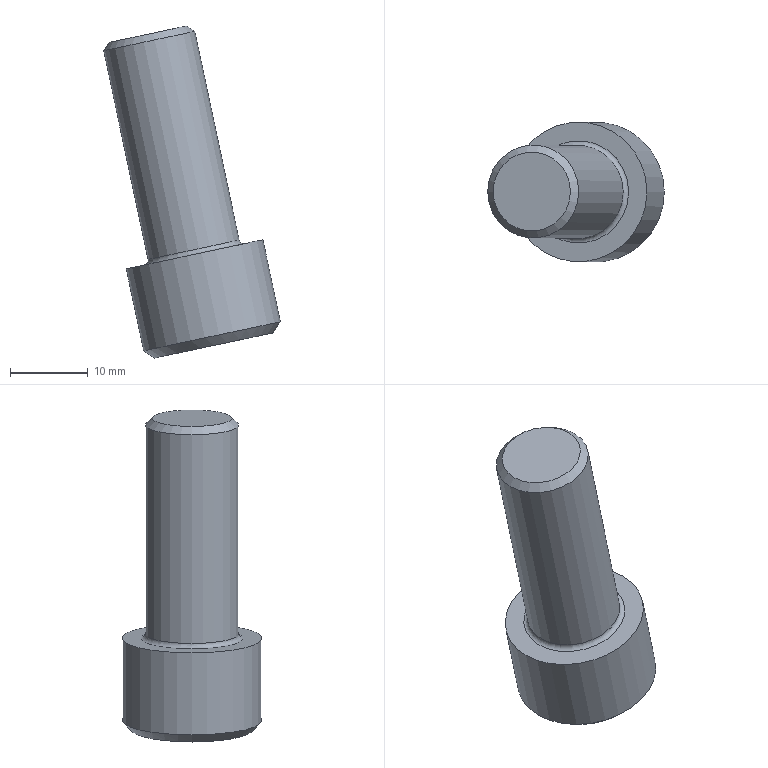Part | STEP file | solid 79 | 1 solid | 21 faces | box 22.76 x 18 x 42.786 mm | volume 5761 mm3 | plane 10 | sphere 6 | cylinder 2 | cone 2 | torus 1 | commonest cylinder face diameters 12 x1 18 x1